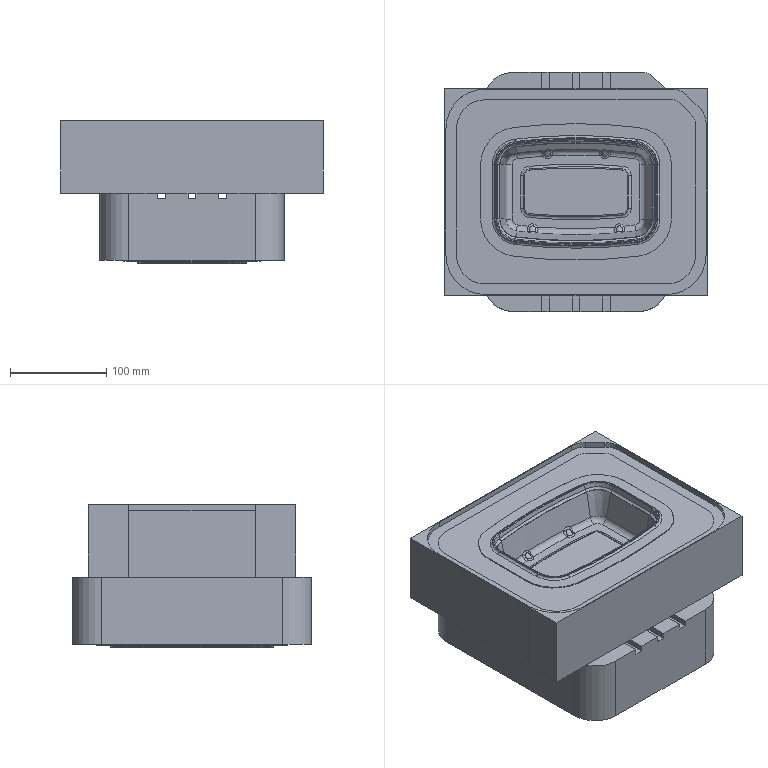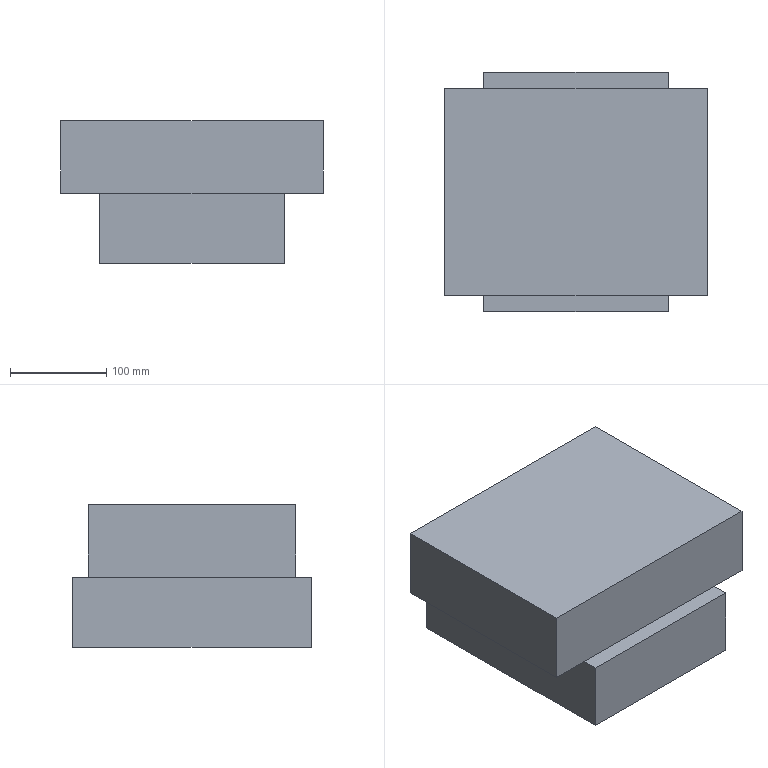CAM job | NX | 3-axis milling, drilling | part box 272.387 x 248.388 x 148.5 mm | stock box 272.387 x 248.387 x 148.5 mm
Tools:
number,name,description,diameter,corner_radius,flute_length,length,flutes
0,V2.0,Drilling Tool,2.0,0.0,35.0,50.0,2
0,V8.0,Drilling Tool,8.0,0.0,35.0,50.0,2
0,D10,No Description,10.0,0.0,20.0,60.0,2
0,D8,No Description,8.0,0.0,0.0,40.0,2
0,D16R0.8,No Description,16.0,0.8,50.0,90.0,2
0,R2,No Description,4.0,2.0,0.0,20.0,2
Operations:
program,operation,operation_type,tool,method,geometry_group,spindle_rpm,surface_speed,feed_per_tooth,feed_cut,feed_plunge,cut_length_mm,path_length_mm,cut_time_min,machine_time_min
B-1,CAVITY_MILL_1,CavityMilling,D16R0.8,METHOD,22B,7000.0,1099.0,0.3214,4500.0,100.0,193569.417,199803.967,43.015,43.639
B-2,CONTOUR_AREA_1,SurfaceContour,R2,METHOD,22B,8000.0,251.0,0.2812,4500.0,100.0,142165.153,142321.441,31.592,31.608
B-2,PLANAR_TEXT_1,Engraving,R2,METHOD,22B,9000.0,113.0,0.0278,500.0,50.0,2144.394,6036.766,8.546,8.935
B-3,DRILLING,Operation,V2.0,METHOD,22B,2000.0,75.0,0.0375,150.0,0.0,220.0,1796.081,1.467,1.624
B-4,FACE_MILLING_1,FaceMilling,D10,METHOD,22B,7000.0,1099.0,0.2857,4000.0,100.0,4794.812,4918.399,1.199,1.211
B-4,PLANAR_MILL_1,PlanarMilling,D10,METHOD,22B,7000.0,571.0,0.1429,2000.0,100.0,81656.241,81850.334,40.828,40.847
C-1,CAVITY_MILL_2,CavityMilling,D8,METHOD,23C,7000.0,1099.0,0.3214,4500.0,100.0,76973.068,92516.054,17.105,18.659
C-2,DRILLING_1,Operation,V2.0,METHOD,23C,2000.0,75.0,0.0375,150.0,0.0,220.0,1703.101,1.467,1.615
C-3,DRILLING_2,Operation,V8.0,METHOD,23C,2000.0,75.0,0.0375,150.0,0.0,987.0,2680.115,6.58,6.749
C-3,DRILLING_2_COPY,Operation,V8.0,METHOD,23C,2000.0,75.0,0.0375,150.0,0.0,184.0,1029.367,1.227,1.311